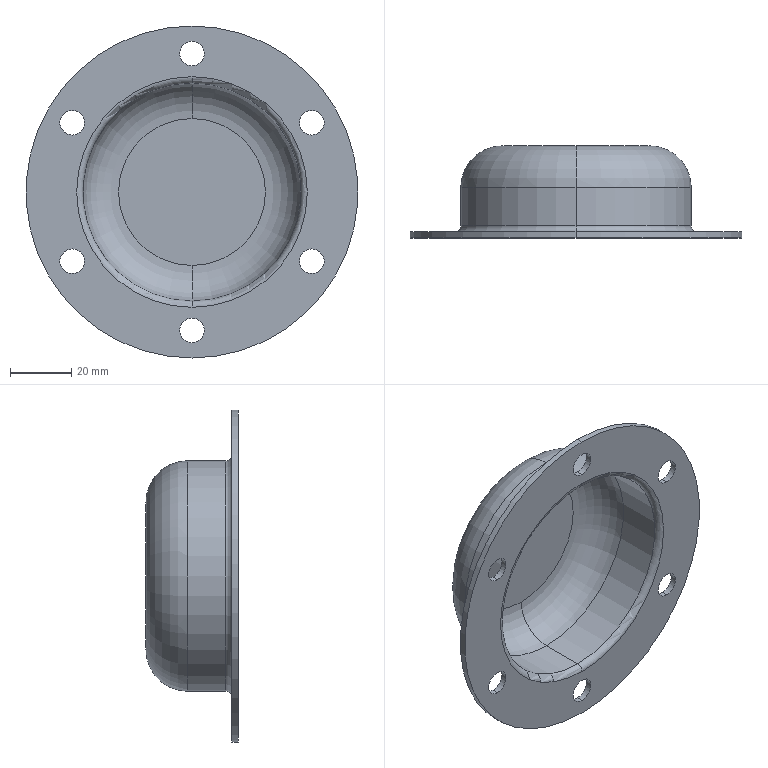Part | SolidWorks | features ICE 1, Revolution 1 | 1 solid | 30 faces | box 108 x 30 x 108 mm | volume 27953 mm3 | cylinder 18 | torus 8 | plane 4 | commonest cylinder face diameters 8 x12 71 x2 75 x2 108 x2
STEP:
#1=CARTESIAN_POINT('',(0.,-15.,-41.));
#2=VERTEX_POINT('',#1);
#3=CARTESIAN_POINT('',(0.,-15.,-49.));
#4=VERTEX_POINT('',#3);
#5=CARTESIAN_POINT('',(0.,-15.,-45.));
#6=DIRECTION('',(0.,-1.,0.));
#7=DIRECTION('',(0.,0.,-1.));
#8=AXIS2_PLACEMENT_3D('',#5,#6,#7);
#9=CIRCLE('',#8,4.);
#10=EDGE_CURVE('',#2,#4,#9,.T.);
#11=ORIENTED_EDGE('',*,*,#10,.T.);
#12=CARTESIAN_POINT('',(0.,-13.,-49.));
#13=VERTEX_POINT('',#12);
#14=CARTESIAN_POINT('',(0.,-23.,-49.));
#15=DIRECTION('',(0.,1.,0.));
#16=VECTOR('',#15,1000.);
#17=LINE('',#14,#16);
#18=EDGE_CURVE('',#4,#13,#17,.T.);
#19=ORIENTED_EDGE('',*,*,#18,.T.);
#20=CARTESIAN_POINT('',(0.,-13.,-41.));
#21=VERTEX_POINT('',#20);
#22=CARTESIAN_POINT('',(0.,-13.,-45.));
#23=DIRECTION('',(0.,1.,0.));
#24=DIRECTION('',(0.,0.,1.));
#25=AXIS2_PLACEMENT_3D('',#22,#23,#24);
#26=CIRCLE('',#25,4.);
#27=EDGE_CURVE('',#13,#21,#26,.T.);
#28=ORIENTED_EDGE('',*,*,#27,.T.);
#29=CARTESIAN_POINT('',(0.,-23.,-41.));
#30=DIRECTION('',(0.,1.,0.));
#31=VECTOR('',#30,1000.);
#32=LINE('',#29,#31);
#33=EDGE_CURVE('',#2,#21,#32,.T.);
#34=ORIENTED_EDGE('',*,*,#33,.F.);
#35=EDGE_LOOP('',(#11,#19,#28,#34));
#36=FACE_OUTER_BOUND('',#35,.T.);
#37=CARTESIAN_POINT('',(0.,-23.,-45.));
#38=DIRECTION('',(0.,1.,0.));
#39=DIRECTION('',(0.,0.,1.));
#40=AXIS2_PLACEMENT_3D('',#37,#38,#39);
#41=CYLINDRICAL_SURFACE('',#40,4.);
#42=ADVANCED_FACE('',(#36),#41,.F.);
#43=CARTESIAN_POINT('',(-38.971,-15.,-18.5));
#44=VERTEX_POINT('',#43);
#45=CARTESIAN_POINT('',(-38.971,-15.,-26.5));
#46=VERTEX_POINT('',#45);
#47=CARTESIAN_POINT('',(-38.971,-15.,-22.5));
#48=DIRECTION('',(0.,-1.,0.));
#49=DIRECTION('',(0.,0.,-1.));
#50=AXIS2_PLACEMENT_3D('',#47,#48,#49);
#51=CIRCLE('',#50,4.);
#52=EDGE_CURVE('',#44,#46,#51,.T.);
#53=ORIENTED_EDGE('',*,*,#52,.T.);
#54=CARTESIAN_POINT('',(-38.971,-13.,-26.5));
#55=VERTEX_POINT('',#54);
#56=CARTESIAN_POINT('',(-38.971,-23.,-26.5));
#57=DIRECTION('',(0.,1.,0.));
#58=VECTOR('',#57,1000.);
#59=LINE('',#56,#58);
#60=EDGE_CURVE('',#46,#55,#59,.T.);
#61=ORIENTED_EDGE('',*,*,#60,.T.);
#62=CARTESIAN_POINT('',(-38.971,-13.,-18.5));
#63=VERTEX_POINT('',#62);
#64=CARTESIAN_POINT('',(-38.971,-13.,-22.5));
#65=DIRECTION('',(0.,1.,0.));
#66=DIRECTION('',(0.,0.,1.));
#67=AXIS2_PLACEMENT_3D('',#64,#65,#66);
#68=CIRCLE('',#67,4.);
#69=EDGE_CURVE('',#55,#63,#68,.T.);
#70=ORIENTED_EDGE('',*,*,#69,.T.);
#71=CARTESIAN_POINT('',(-38.971,-23.,-18.5));
#72=DIRECTION('',(0.,1.,0.));
#73=VECTOR('',#72,1000.);
#74=LINE('',#71,#73);
#75=EDGE_CURVE('',#44,#63,#74,.T.);
#76=ORIENTED_EDGE('',*,*,#75,.F.);
#77=EDGE_LOOP('',(#53,#61,#70,#76));
#78=FACE_OUTER_BOUND('',#77,.T.);
#79=CARTESIAN_POINT('',(-38.971,-23.,-22.5));
#80=DIRECTION('',(0.,1.,0.));
#81=DIRECTION('',(0.,0.,1.));
#82=AXIS2_PLACEMENT_3D('',#79,#80,#81);
#83=CYLINDRICAL_SURFACE('',#82,4.);
#84=ADVANCED_FACE('',(#78),#83,.F.);
#85=CARTESIAN_POINT('',(-38.971,-15.,26.5));
#86=VERTEX_POINT('',#85);
#87=CARTESIAN_POINT('',(-38.971,-15.,18.5));
#88=VERTEX_POINT('',#87);
#89=CARTESIAN_POINT('',(-38.971,-15.,22.5));
#90=DIRECTION('',(0.,-1.,0.));
#91=DIRECTION('',(0.,0.,-1.));
#92=AXIS2_PLACEMENT_3D('',#89,#90,#91);
#93=CIRCLE('',#92,4.);
#94=EDGE_CURVE('',#86,#88,#93,.T.);
#95=ORIENTED_EDGE('',*,*,#94,.T.);
#96=CARTESIAN_POINT('',(-38.971,-13.,18.5));
#97=VERTEX_POINT('',#96);
#98=CARTESIAN_POINT('',(-38.971,-23.,18.5));
#99=DIRECTION('',(0.,1.,0.));
#100=VECTOR('',#99,1000.);
#101=LINE('',#98,#100);
#102=EDGE_CURVE('',#88,#97,#101,.T.);
#103=ORIENTED_EDGE('',*,*,#102,.T.);
#104=CARTESIAN_POINT('',(-38.971,-13.,26.5));
#105=VERTEX_POINT('',#104);
#106=CARTESIAN_POINT('',(-38.971,-13.,22.5));
#107=DIRECTION('',(0.,1.,0.));
#108=DIRECTION('',(0.,0.,1.));
#109=AXIS2_PLACEMENT_3D('',#106,#107,#108);
#110=CIRCLE('',#109,4.);
#111=EDGE_CURVE('',#97,#105,#110,.T.);
#112=ORIENTED_EDGE('',*,*,#111,.T.);
#113=CARTESIAN_POINT('',(-38.971,-23.,26.5));
#114=DIRECTION('',(0.,1.,0.));
#115=VECTOR('',#114,1000.);
#116=LINE('',#113,#115);
#117=EDGE_CURVE('',#86,#105,#116,.T.);
#118=ORIENTED_EDGE('',*,*,#117,.F.);
#119=EDGE_LOOP('',(#95,#103,#112,#118));
#120=FACE_OUTER_BOUND('',#119,.T.);
#121=CARTESIAN_POINT('',(-38.971,-23.,22.5));
#122=DIRECTION('',(0.,1.,0.));
#123=DIRECTION('',(0.,0.,1.));
#124=AXIS2_PLACEMENT_3D('',#121,#122,#123);
#125=CYLINDRICAL_SURFACE('',#124,4.);
#126=ADVANCED_FACE('',(#120),#125,.F.);
#127=CARTESIAN_POINT('',(0.,-15.,49.));
#128=VERTEX_POINT('',#127);
#129=CARTESIAN_POINT('',(0.,-15.,41.));
#130=VERTEX_POINT('',#129);
#131=CARTESIAN_POINT('',(0.,-15.,45.));
#132=DIRECTION('',(0.,-1.,0.));
#133=DIRECTION('',(0.,0.,-1.));
#134=AXIS2_PLACEMENT_3D('',#131,#132,#133);
#135=CIRCLE('',#134,4.);
#136=EDGE_CURVE('',#128,#130,#135,.T.);
#137=ORIENTED_EDGE('',*,*,#136,.T.);
#138=CARTESIAN_POINT('',(0.,-13.,41.));
#139=VERTEX_POINT('',#138);
#140=CARTESIAN_POINT('',(0.,-23.,41.));
#141=DIRECTION('',(0.,1.,0.));
#142=VECTOR('',#141,1000.);
#143=LINE('',#140,#142);
#144=EDGE_CURVE('',#130,#139,#143,.T.);
#145=ORIENTED_EDGE('',*,*,#144,.T.);
#146=CARTESIAN_POINT('',(0.,-13.,49.));
#147=VERTEX_POINT('',#146);
#148=CARTESIAN_POINT('',(0.,-13.,45.));
#149=DIRECTION('',(0.,1.,0.));
#150=DIRECTION('',(0.,0.,1.));
#151=AXIS2_PLACEMENT_3D('',#148,#149,#150);
#152=CIRCLE('',#151,4.);
#153=EDGE_CURVE('',#139,#147,#152,.T.);
#154=ORIENTED_EDGE('',*,*,#153,.T.);
#155=CARTESIAN_POINT('',(0.,-23.,49.));
#156=DIRECTION('',(0.,1.,0.));
#157=VECTOR('',#156,1000.);
#158=LINE('',#155,#157);
#159=EDGE_CURVE('',#128,#147,#158,.T.);
#160=ORIENTED_EDGE('',*,*,#159,.F.);
#161=EDGE_LOOP('',(#137,#145,#154,#160));
#162=FACE_OUTER_BOUND('',#161,.T.);
#163=CARTESIAN_POINT('',(0.,-23.,45.));
#164=DIRECTION('',(0.,1.,0.));
#165=DIRECTION('',(0.,0.,1.));
#166=AXIS2_PLACEMENT_3D('',#163,#164,#165);
#167=CYLINDRICAL_SURFACE('',#166,4.);
#168=ADVANCED_FACE('',(#162),#167,.F.);
#169=CARTESIAN_POINT('',(38.971,-15.,26.5));
#170=VERTEX_POINT('',#169);
#171=CARTESIAN_POINT('',(38.971,-15.,18.5));
#172=VERTEX_POINT('',#171);
#173=CARTESIAN_POINT('',(38.971,-15.,22.5));
#174=DIRECTION('',(0.,-1.,0.));
#175=DIRECTION('',(0.,0.,-1.));
#176=AXIS2_PLACEMENT_3D('',#173,#174,#175);
#177=CIRCLE('',#176,4.);
#178=EDGE_CURVE('',#170,#172,#177,.T.);
#179=ORIENTED_EDGE('',*,*,#178,.T.);
#180=CARTESIAN_POINT('',(38.971,-13.,18.5));
#181=VERTEX_POINT('',#180);
#182=CARTESIAN_POINT('',(38.971,-23.,18.5));
#183=DIRECTION('',(0.,1.,0.));
#184=VECTOR('',#183,1000.);
#185=LINE('',#182,#184);
#186=EDGE_CURVE('',#172,#181,#185,.T.);
#187=ORIENTED_EDGE('',*,*,#186,.T.);
#188=CARTESIAN_POINT('',(38.971,-13.,26.5));
#189=VERTEX_POINT('',#188);
#190=CARTESIAN_POINT('',(38.971,-13.,22.5));
#191=DIRECTION('',(0.,1.,0.));
#192=DIRECTION('',(0.,0.,1.));
#193=AXIS2_PLACEMENT_3D('',#190,#191,#192);
#194=CIRCLE('',#193,4.);
#195=EDGE_CURVE('',#181,#189,#194,.T.);
#196=ORIENTED_EDGE('',*,*,#195,.T.);
#197=CARTESIAN_POINT('',(38.971,-23.,26.5));
#198=DIRECTION('',(0.,1.,0.));
#199=VECTOR('',#198,1000.);
#200=LINE('',#197,#199);
#201=EDGE_CURVE('',#170,#189,#200,.T.);
#202=ORIENTED_EDGE('',*,*,#201,.F.);
#203=EDGE_LOOP('',(#179,#187,#196,#202));
#204=FACE_OUTER_BOUND('',#203,.T.);
#205=CARTESIAN_POINT('',(38.971,-23.,22.5));
#206=DIRECTION('',(0.,1.,0.));
#207=DIRECTION('',(0.,0.,1.));
#208=AXIS2_PLACEMENT_3D('',#205,#206,#207);
#209=CYLINDRICAL_SURFACE('',#208,4.);
#210=ADVANCED_FACE('',(#204),#209,.F.);
#211=CARTESIAN_POINT('',(38.971,-15.,-18.5));
#212=VERTEX_POINT('',#211);
#213=CARTESIAN_POINT('',(38.971,-15.,-26.5));
#214=VERTEX_POINT('',#213);
#215=CARTESIAN_POINT('',(38.971,-15.,-22.5));
#216=DIRECTION('',(0.,-1.,0.));
#217=DIRECTION('',(0.,0.,-1.));
#218=AXIS2_PLACEMENT_3D('',#215,#216,#217);
#219=CIRCLE('',#218,4.);
#220=EDGE_CURVE('',#212,#214,#219,.T.);
#221=ORIENTED_EDGE('',*,*,#220,.T.);
#222=CARTESIAN_POINT('',(38.971,-13.,-26.5));
#223=VERTEX_POINT('',#222);
#224=CARTESIAN_POINT('',(38.971,-23.,-26.5));
#225=DIRECTION('',(0.,1.,0.));
#226=VECTOR('',#225,1000.);
#227=LINE('',#224,#226);
#228=EDGE_CURVE('',#214,#223,#227,.T.);
#229=ORIENTED_EDGE('',*,*,#228,.T.);
#230=CARTESIAN_POINT('',(38.971,-13.,-18.5));
#231=VERTEX_POINT('',#230);
#232=CARTESIAN_POINT('',(38.971,-13.,-22.5));
#233=DIRECTION('',(0.,1.,0.));
#234=DIRECTION('',(0.,0.,1.));
#235=AXIS2_PLACEMENT_3D('',#232,#233,#234);
#236=CIRCLE('',#235,4.);
#237=EDGE_CURVE('',#223,#231,#236,.T.);
#238=ORIENTED_EDGE('',*,*,#237,.T.);
#239=CARTESIAN_POINT('',(38.971,-23.,-18.5));
#240=DIRECTION('',(0.,1.,0.));
#241=VECTOR('',#240,1000.);
#242=LINE('',#239,#241);
#243=EDGE_CURVE('',#212,#231,#242,.T.);
#244=ORIENTED_EDGE('',*,*,#243,.F.);
#245=EDGE_LOOP('',(#221,#229,#238,#244));
#246=FACE_OUTER_BOUND('',#245,.T.);
#247=CARTESIAN_POINT('',(38.971,-23.,-22.5));
#248=DIRECTION('',(0.,1.,0.));
#249=DIRECTION('',(0.,0.,1.));
#250=AXIS2_PLACEMENT_3D('',#247,#248,#249);
#251=CYLINDRICAL_SURFACE('',#250,4.);
#252=ADVANCED_FACE('',(#246),#251,.F.);
#253=CARTESIAN_POINT('',(0.,1.423,-37.5));
#254=VERTEX_POINT('',#253);
#255=CARTESIAN_POINT('',(0.,1.423,37.5));
#256=VERTEX_POINT('',#255);
#257=CARTESIAN_POINT('',(0.,1.423,0.));
#258=DIRECTION('',(0.,-1.,0.));
#259=DIRECTION('',(0.,0.,-1.));
#260=AXIS2_PLACEMENT_3D('',#257,#258,#259);
#261=CIRCLE('',#260,37.5);
#262=EDGE_CURVE('',#254,#256,#261,.T.);
#263=ORIENTED_EDGE('',*,*,#262,.T.);
#264=CARTESIAN_POINT('',(0.,-11.,37.5));
#265=VERTEX_POINT('',#264);
#266=CARTESIAN_POINT('',(0.,0.,37.5));
#267=DIRECTION('',(0.,-1.,0.));
#268=VECTOR('',#267,1000.);
#269=LINE('',#266,#268);
#270=EDGE_CURVE('',#256,#265,#269,.T.);
#271=ORIENTED_EDGE('',*,*,#270,.T.);
#272=CARTESIAN_POINT('',(0.,-11.,-37.5));
#273=VERTEX_POINT('',#272);
#274=CARTESIAN_POINT('',(0.,-11.,0.));
#275=DIRECTION('',(0.,-1.,0.));
#276=DIRECTION('',(0.,0.,-1.));
#277=AXIS2_PLACEMENT_3D('',#274,#275,#276);
#278=CIRCLE('',#277,37.5);
#279=EDGE_CURVE('',#273,#265,#278,.T.);
#280=ORIENTED_EDGE('',*,*,#279,.F.);
#281=CARTESIAN_POINT('',(0.,0.,-37.5));
#282=DIRECTION('',(0.,-1.,0.));
#283=VECTOR('',#282,1000.);
#284=LINE('',#281,#283);
#285=EDGE_CURVE('',#254,#273,#284,.T.);
#286=ORIENTED_EDGE('',*,*,#285,.F.);
#287=EDGE_LOOP('',(#263,#271,#280,#286));
#288=FACE_OUTER_BOUND('',#287,.T.);
#289=CARTESIAN_POINT('',(0.,0.,0.));
#290=DIRECTION('',(0.,-1.,0.));
#291=DIRECTION('',(0.,0.,-1.));
#292=AXIS2_PLACEMENT_3D('',#289,#290,#291);
#293=CYLINDRICAL_SURFACE('',#292,37.5);
#294=ADVANCED_FACE('',(#288),#293,.T.);
#295=CARTESIAN_POINT('',(0.,-13.,39.5));
#296=VERTEX_POINT('',#295);
#297=CARTESIAN_POINT('',(0.,-13.,-39.5));
#298=VERTEX_POINT('',#297);
#299=CARTESIAN_POINT('',(0.,-13.,0.));
#300=DIRECTION('',(0.,-1.,0.));
#301=DIRECTION('',(0.,0.,-1.));
#302=AXIS2_PLACEMENT_3D('',#299,#300,#301);
#303=CIRCLE('',#302,39.5);
#304=EDGE_CURVE('',#296,#298,#303,.T.);
#305=ORIENTED_EDGE('',*,*,#304,.F.);
#306=CARTESIAN_POINT('',(0.,-11.,39.5));
#307=DIRECTION('',(1.,0.,0.));
#308=DIRECTION('',(0.,0.,-1.));
#309=AXIS2_PLACEMENT_3D('',#306,#307,#308);
#310=CIRCLE('',#309,2.);
#311=EDGE_CURVE('',#296,#265,#310,.T.);
#312=ORIENTED_EDGE('',*,*,#311,.T.);
#313=CARTESIAN_POINT('',(0.,-11.,0.));
#314=DIRECTION('',(0.,-1.,0.));
#315=DIRECTION('',(0.,0.,-1.));
#316=AXIS2_PLACEMENT_3D('',#313,#314,#315);
#317=CIRCLE('',#316,37.5);
#318=EDGE_CURVE('',#265,#273,#317,.T.);
#319=ORIENTED_EDGE('',*,*,#318,.T.);
#320=CARTESIAN_POINT('',(0.,-11.,-39.5));
#321=DIRECTION('',(-1.,0.,0.));
#322=DIRECTION('',(0.,0.,1.));
#323=AXIS2_PLACEMENT_3D('',#320,#321,#322);
#324=CIRCLE('',#323,2.);
#325=EDGE_CURVE('',#298,#273,#324,.T.);
#326=ORIENTED_EDGE('',*,*,#325,.F.);
#327=EDGE_LOOP('',(#305,#312,#319,#326));
#328=FACE_OUTER_BOUND('',#327,.T.);
#329=CARTESIAN_POINT('',(0.,-11.,0.));
#330=DIRECTION('',(0.,-1.,0.));
#331=DIRECTION('',(0.,0.,-1.));
#332=AXIS2_PLACEMENT_3D('',#329,#330,#331);
#333=TOROIDAL_SURFACE('',#332,39.5,2.);
#334=ADVANCED_FACE('',(#328),#333,.F.);
#335=CARTESIAN_POINT('',(0.,-13.,-54.));
#336=VERTEX_POINT('',#335);
#337=CARTESIAN_POINT('',(0.,-13.,54.));
#338=VERTEX_POINT('',#337);
#339=CARTESIAN_POINT('',(0.,-13.,0.));
#340=DIRECTION('',(0.,-1.,0.));
#341=DIRECTION('',(0.,0.,-1.));
#342=AXIS2_PLACEMENT_3D('',#339,#340,#341);
#343=CIRCLE('',#342,54.);
#344=EDGE_CURVE('',#336,#338,#343,.T.);
#345=ORIENTED_EDGE('',*,*,#344,.T.);
#346=CARTESIAN_POINT('',(0.,-15.,54.));
#347=VERTEX_POINT('',#346);
#348=CARTESIAN_POINT('',(0.,0.,54.));
#349=DIRECTION('',(0.,-1.,0.));
#350=VECTOR('',#349,1000.);
#351=LINE('',#348,#350);
#352=EDGE_CURVE('',#338,#347,#351,.T.);
#353=ORIENTED_EDGE('',*,*,#352,.T.);
#354=CARTESIAN_POINT('',(0.,-15.,-54.));
#355=VERTEX_POINT('',#354);
#356=CARTESIAN_POINT('',(0.,-15.,0.));
#357=DIRECTION('',(0.,-1.,0.));
#358=DIRECTION('',(0.,0.,-1.));
#359=AXIS2_PLACEMENT_3D('',#356,#357,#358);
#360=CIRCLE('',#359,54.);
#361=EDGE_CURVE('',#355,#347,#360,.T.);
#362=ORIENTED_EDGE('',*,*,#361,.F.);
#363=CARTESIAN_POINT('',(0.,0.,-54.));
#364=DIRECTION('',(0.,-1.,0.));
#365=VECTOR('',#364,1000.);
#366=LINE('',#363,#365);
#367=EDGE_CURVE('',#336,#355,#366,.T.);
#368=ORIENTED_EDGE('',*,*,#367,.F.);
#369=EDGE_LOOP('',(#345,#353,#362,#368));
#370=FACE_OUTER_BOUND('',#369,.T.);
#371=CARTESIAN_POINT('',(0.,0.,0.));
#372=DIRECTION('',(0.,-1.,0.));
#373=DIRECTION('',(0.,0.,-1.));
#374=AXIS2_PLACEMENT_3D('',#371,#372,#373);
#375=CYLINDRICAL_SURFACE('',#374,54.);
#376=ADVANCED_FACE('',(#370),#375,.T.);
#377=CARTESIAN_POINT('',(0.,-15.,-37.5));
#378=VERTEX_POINT('',#377);
#379=CARTESIAN_POINT('',(0.,-15.,37.5));
#380=VERTEX_POINT('',#379);
#381=CARTESIAN_POINT('',(0.,-15.,0.));
#382=DIRECTION('',(0.,-1.,0.));
#383=DIRECTION('',(0.,0.,-1.));
#384=AXIS2_PLACEMENT_3D('',#381,#382,#383);
#385=CIRCLE('',#384,37.5);
#386=EDGE_CURVE('',#378,#380,#385,.T.);
#387=ORIENTED_EDGE('',*,*,#386,.T.);
#388=CARTESIAN_POINT('',(0.,-13.,35.5));
#389=VERTEX_POINT('',#388);
#390=CARTESIAN_POINT('',(0.,-13.,37.5));
#391=DIRECTION('',(1.,0.,0.));
#392=DIRECTION('',(0.,0.,-1.));
#393=AXIS2_PLACEMENT_3D('',#390,#391,#392);
#394=CIRCLE('',#393,2.);
#395=EDGE_CURVE('',#380,#389,#394,.T.);
#396=ORIENTED_EDGE('',*,*,#395,.T.);
#397=CARTESIAN_POINT('',(0.,-13.,-35.5));
#398=VERTEX_POINT('',#397);
#399=CARTESIAN_POINT('',(0.,-13.,0.));
#400=DIRECTION('',(0.,-1.,0.));
#401=DIRECTION('',(0.,0.,-1.));
#402=AXIS2_PLACEMENT_3D('',#399,#400,#401);
#403=CIRCLE('',#402,35.5);
#404=EDGE_CURVE('',#398,#389,#403,.T.);
#405=ORIENTED_EDGE('',*,*,#404,.F.);
#406=CARTESIAN_POINT('',(0.,-13.,-37.5));
#407=DIRECTION('',(-1.,0.,0.));
#408=DIRECTION('',(0.,0.,1.));
#409=AXIS2_PLACEMENT_3D('',#406,#407,#408);
#410=CIRCLE('',#409,2.);
#411=EDGE_CURVE('',#378,#398,#410,.T.);
#412=ORIENTED_EDGE('',*,*,#411,.F.);
#413=EDGE_LOOP('',(#387,#396,#405,#412));
#414=FACE_OUTER_BOUND('',#413,.T.);
#415=CARTESIAN_POINT('',(0.,-13.,0.));
#416=DIRECTION('',(0.,-1.,0.));
#417=DIRECTION('',(0.,0.,-1.));
#418=AXIS2_PLACEMENT_3D('',#415,#416,#417);
#419=TOROIDAL_SURFACE('',#418,37.5,2.);
#420=ADVANCED_FACE('',(#414),#419,.T.);
#421=CARTESIAN_POINT('',(0.,1.423,35.5));
#422=VERTEX_POINT('',#421);
#423=CARTESIAN_POINT('',(0.,1.423,-35.5));
#424=VERTEX_POINT('',#423);
#425=CARTESIAN_POINT('',(0.,1.423,0.));
#426=DIRECTION('',(0.,-1.,0.));
#427=DIRECTION('',(0.,0.,-1.));
#428=AXIS2_PLACEMENT_3D('',#425,#426,#427);
#429=CIRCLE('',#428,35.5);
#430=EDGE_CURVE('',#422,#424,#429,.T.);
#431=ORIENTED_EDGE('',*,*,#430,.F.);
#432=CARTESIAN_POINT('',(0.,0.,35.5));
#433=DIRECTION('',(0.,-1.,0.));
#434=VECTOR('',#433,1000.);
#435=LINE('',#432,#434);
#436=EDGE_CURVE('',#422,#389,#435,.T.);
#437=ORIENTED_EDGE('',*,*,#436,.T.);
#438=CARTESIAN_POINT('',(0.,-13.,0.));
#439=DIRECTION('',(0.,-1.,0.));
#440=DIRECTION('',(0.,0.,-1.));
#441=AXIS2_PLACEMENT_3D('',#438,#439,#440);
#442=CIRCLE('',#441,35.5);
#443=EDGE_CURVE('',#389,#398,#442,.T.);
#444=ORIENTED_EDGE('',*,*,#443,.T.);
#445=CARTESIAN_POINT('',(0.,0.,-35.5));
#446=DIRECTION('',(0.,-1.,0.));
#447=VECTOR('',#446,1000.);
#448=LINE('',#445,#447);
#449=EDGE_CURVE('',#424,#398,#448,.T.);
#450=ORIENTED_EDGE('',*,*,#449,.F.);
#451=EDGE_LOOP('',(#431,#437,#444,#450));
#452=FACE_OUTER_BOUND('',#451,.T.);
#453=CARTESIAN_POINT('',(0.,0.,0.));
#454=DIRECTION('',(0.,-1.,0.));
#455=DIRECTION('',(0.,0.,-1.));
#456=AXIS2_PLACEMENT_3D('',#453,#454,#455);
#457=CYLINDRICAL_SURFACE('',#456,35.5);
#458=ADVANCED_FACE('',(#452),#457,.F.);
#459=CARTESIAN_POINT('',(0.,13.,23.923));
#460=VERTEX_POINT('',#459);
#461=CARTESIAN_POINT('',(0.,13.,-23.923));
#462=VERTEX_POINT('',#461);
#463=CARTESIAN_POINT('',(0.,13.,0.));
#464=DIRECTION('',(0.,-1.,0.));
#465=DIRECTION('',(0.,0.,-1.));
#466=AXIS2_PLACEMENT_3D('',#463,#464,#465);
#467=CIRCLE('',#466,23.923);
#468=EDGE_CURVE('',#460,#462,#467,.T.);
#469=ORIENTED_EDGE('',*,*,#468,.F.);
#470=CARTESIAN_POINT('',(0.,1.423,23.923));
#471=DIRECTION('',(1.,0.,0.));
#472=DIRECTION('',(0.,0.,-1.));
#473=AXIS2_PLACEMENT_3D('',#470,#471,#472);
#474=CIRCLE('',#473,11.577);
#475=EDGE_CURVE('',#460,#422,#474,.T.);
#476=ORIENTED_EDGE('',*,*,#475,.T.);
#477=ORIENTED_EDGE('',*,*,#430,.T.);
#478=CARTESIAN_POINT('',(0.,1.423,-23.923));
#479=DIRECTION('',(-1.,0.,0.));
#480=DIRECTION('',(0.,0.,1.));
#481=AXIS2_PLACEMENT_3D('',#478,#479,#480);
#482=CIRCLE('',#481,11.577);
#483=EDGE_CURVE('',#462,#424,#482,.T.);
#484=ORIENTED_EDGE('',*,*,#483,.F.);
#485=EDGE_LOOP('',(#469,#476,#477,#484));
#486=FACE_OUTER_BOUND('',#485,.T.);
#487=CARTESIAN_POINT('',(0.,1.423,0.));
#488=DIRECTION('',(0.,-1.,0.));
#489=DIRECTION('',(0.,0.,-1.));
#490=AXIS2_PLACEMENT_3D('',#487,#488,#489);
#491=TOROIDAL_SURFACE('',#490,23.923,11.577);
#492=ADVANCED_FACE('',(#486),#491,.F.);
#493=CARTESIAN_POINT('',(0.,15.,-23.923));
#494=VERTEX_POINT('',#493);
#495=CARTESIAN_POINT('',(0.,15.,23.923));
#496=VERTEX_POINT('',#495);
#497=CARTESIAN_POINT('',(0.,15.,0.));
#498=DIRECTION('',(0.,-1.,0.));
#499=DIRECTION('',(0.,0.,-1.));
#500=AXIS2_PLACEMENT_3D('',#497,#498,#499);
#501=CIRCLE('',#500,23.923);
#502=EDGE_CURVE('',#494,#496,#501,.T.);
#503=ORIENTED_EDGE('',*,*,#502,.T.);
#504=CARTESIAN_POINT('',(0.,1.423,23.923));
#505=DIRECTION('',(1.,0.,0.));
#506=DIRECTION('',(0.,0.,-1.));
#507=AXIS2_PLACEMENT_3D('',#504,#505,#506);
#508=CIRCLE('',#507,13.577);
#509=EDGE_CURVE('',#496,#256,#508,.T.);
#510=ORIENTED_EDGE('',*,*,#509,.T.);
#511=ORIENTED_EDGE('',*,*,#262,.F.);
#512=CARTESIAN_POINT('',(0.,1.423,-23.923));
#513=DIRECTION('',(-1.,0.,0.));
#514=DIRECTION('',(0.,0.,1.));
#515=AXIS2_PLACEMENT_3D('',#512,#513,#514);
#516=CIRCLE('',#515,13.577);
#517=EDGE_CURVE('',#494,#254,#516,.T.);
#518=ORIENTED_EDGE('',*,*,#517,.F.);
#519=EDGE_LOOP('',(#503,#510,#511,#518));
#520=FACE_OUTER_BOUND('',#519,.T.);
#521=CARTESIAN_POINT('',(0.,1.423,0.));
#522=DIRECTION('',(0.,-1.,0.));
#523=DIRECTION('',(0.,0.,-1.));
#524=AXIS2_PLACEMENT_3D('',#521,#522,#523);
#525=TOROIDAL_SURFACE('',#524,23.923,13.577);
#526=ADVANCED_FACE('',(#520),#525,.T.);
#527=ORIENTED_EDGE('',*,*,#509,.F.);
#528=CARTESIAN_POINT('',(0.,15.,0.));
#529=DIRECTION('',(0.,-1.,0.));
#530=DIRECTION('',(0.,0.,-1.));
#531=AXIS2_PLACEMENT_3D('',#528,#529,#530);
#532=CIRCLE('',#531,23.923);
#533=EDGE_CURVE('',#496,#494,#532,.T.);
#534=ORIENTED_EDGE('',*,*,#533,.T.);
#535=ORIENTED_EDGE('',*,*,#517,.T.);
#536=CARTESIAN_POINT('',(0.,1.423,0.));
#537=DIRECTION('',(0.,-1.,0.));
#538=DIRECTION('',(0.,0.,-1.));
#539=AXIS2_PLACEMENT_3D('',#536,#537,#538);
#540=CIRCLE('',#539,37.5);
#541=EDGE_CURVE('',#256,#254,#540,.T.);
#542=ORIENTED_EDGE('',*,*,#541,.F.);
#543=EDGE_LOOP('',(#527,#534,#535,#542));
#544=FACE_OUTER_BOUND('',#543,.T.);
#545=CARTESIAN_POINT('',(0.,1.423,0.));
#546=DIRECTION('',(0.,-1.,0.));
#547=DIRECTION('',(0.,0.,-1.));
#548=AXIS2_PLACEMENT_3D('',#545,#546,#547);
#549=TOROIDAL_SURFACE('',#548,23.923,13.577);
#550=ADVANCED_FACE('',(#544),#549,.T.);
#551=ORIENTED_EDGE('',*,*,#502,.F.);
#552=ORIENTED_EDGE('',*,*,#533,.F.);
#553=EDGE_LOOP('',(#551,#552));
#554=FACE_OUTER_BOUND('',#553,.T.);
#555=CARTESIAN_POINT('',(23.923,15.,0.));
#556=DIRECTION('',(0.,1.,0.));
#557=DIRECTION('',(0.,0.,1.));
#558=AXIS2_PLACEMENT_3D('',#555,#556,#557);
#559=PLANE('',#558);
#560=ADVANCED_FACE('',(#554),#559,.T.);
#561=CARTESIAN_POINT('',(0.,13.,0.));
#562=DIRECTION('',(0.,-1.,0.));
#563=DIRECTION('',(0.,0.,-1.));
#564=AXIS2_PLACEMENT_3D('',#561,#562,#563);
#565=CIRCLE('',#564,23.923);
#566=EDGE_CURVE('',#462,#460,#565,.T.);
#567=ORIENTED_EDGE('',*,*,#566,.T.);
#568=ORIENTED_EDGE('',*,*,#468,.T.);
#569=EDGE_LOOP('',(#567,#568));
#570=FACE_OUTER_BOUND('',#569,.T.);
#571=CARTESIAN_POINT('',(0.,13.,0.));
#572=DIRECTION('',(0.,-1.,0.));
#573=DIRECTION('',(0.,0.,-1.));
#574=AXIS2_PLACEMENT_3D('',#571,#572,#573);
#575=PLANE('',#574);
#576=ADVANCED_FACE('',(#570),#575,.T.);
#577=ORIENTED_EDGE('',*,*,#475,.F.);
#578=ORIENTED_EDGE('',*,*,#566,.F.);
#579=ORIENTED_EDGE('',*,*,#483,.T.);
#580=CARTESIAN_POINT('',(0.,1.423,0.));
#581=DIRECTION('',(0.,-1.,0.));
#582=DIRECTION('',(0.,0.,-1.));
#583=AXIS2_PLACEMENT_3D('',#580,#581,#582);
#584=CIRCLE('',#583,35.5);
#585=EDGE_CURVE('',#424,#422,#584,.T.);
#586=ORIENTED_EDGE('',*,*,#585,.T.);
#587=EDGE_LOOP('',(#577,#578,#579,#586));
#588=FACE_OUTER_BOUND('',#587,.T.);
#589=CARTESIAN_POINT('',(0.,1.423,0.));
#590=DIRECTION('',(0.,-1.,0.));
#591=DIRECTION('',(0.,0.,-1.));
#592=AXIS2_PLACEMENT_3D('',#589,#590,#591);
#593=TOROIDAL_SURFACE('',#592,23.923,11.577);
#594=ADVANCED_FACE('',(#588),#593,.F.);
#595=ORIENTED_EDGE('',*,*,#436,.F.);
#596=ORIENTED_EDGE('',*,*,#585,.F.);
#597=ORIENTED_EDGE('',*,*,#449,.T.);
#598=ORIENTED_EDGE('',*,*,#404,.T.);
#599=EDGE_LOOP('',(#595,#596,#597,#598));
#600=FACE_OUTER_BOUND('',#599,.T.);
#601=CARTESIAN_POINT('',(0.,0.,0.));
#602=DIRECTION('',(0.,-1.,0.));
#603=DIRECTION('',(0.,0.,-1.));
#604=AXIS2_PLACEMENT_3D('',#601,#602,#603);
#605=CYLINDRICAL_SURFACE('',#604,35.5);
#606=ADVANCED_FACE('',(#600),#605,.F.);
#607=ORIENTED_EDGE('',*,*,#395,.F.);
#608=CARTESIAN_POINT('',(0.,-15.,0.));
#609=DIRECTION('',(0.,-1.,0.));
#610=DIRECTION('',(0.,0.,-1.));
#611=AXIS2_PLACEMENT_3D('',#608,#609,#610);
#612=CIRCLE('',#611,37.5);
#613=EDGE_CURVE('',#380,#378,#612,.T.);
#614=ORIENTED_EDGE('',*,*,#613,.T.);
#615=ORIENTED_EDGE('',*,*,#411,.T.);
#616=ORIENTED_EDGE('',*,*,#443,.F.);
#617=EDGE_LOOP('',(#607,#614,#615,#616));
#618=FACE_OUTER_BOUND('',#617,.T.);
#619=CARTESIAN_POINT('',(0.,-13.,0.));
#620=DIRECTION('',(0.,-1.,0.));
#621=DIRECTION('',(0.,0.,-1.));
#622=AXIS2_PLACEMENT_3D('',#619,#620,#621);
#623=TOROIDAL_SURFACE('',#622,37.5,2.);
#624=ADVANCED_FACE('',(#618),#623,.T.);
#625=ORIENTED_EDGE('',*,*,#10,.F.);
#626=CARTESIAN_POINT('',(0.,-15.,-45.));
#627=DIRECTION('',(0.,-1.,0.));
#628=DIRECTION('',(0.,0.,-1.));
#629=AXIS2_PLACEMENT_3D('',#626,#627,#628);
#630=CIRCLE('',#629,4.);
#631=EDGE_CURVE('',#4,#2,#630,.T.);
#632=ORIENTED_EDGE('',*,*,#631,.F.);
#633=EDGE_LOOP('',(#625,#632));
#634=FACE_BOUND('',#633,.T.);
#635=ORIENTED_EDGE('',*,*,#52,.F.);
#636=CARTESIAN_POINT('',(-38.971,-15.,-22.5));
#637=DIRECTION('',(0.,-1.,0.));
#638=DIRECTION('',(0.,0.,-1.));
#639=AXIS2_PLACEMENT_3D('',#636,#637,#638);
#640=CIRCLE('',#639,4.);
#641=EDGE_CURVE('',#46,#44,#640,.T.);
#642=ORIENTED_EDGE('',*,*,#641,.F.);
#643=EDGE_LOOP('',(#635,#642));
#644=FACE_BOUND('',#643,.T.);
#645=ORIENTED_EDGE('',*,*,#94,.F.);
#646=CARTESIAN_POINT('',(-38.971,-15.,22.5));
#647=DIRECTION('',(0.,-1.,0.));
#648=DIRECTION('',(0.,0.,-1.));
#649=AXIS2_PLACEMENT_3D('',#646,#647,#648);
#650=CIRCLE('',#649,4.);
#651=EDGE_CURVE('',#88,#86,#650,.T.);
#652=ORIENTED_EDGE('',*,*,#651,.F.);
#653=EDGE_LOOP('',(#645,#652));
#654=FACE_BOUND('',#653,.T.);
#655=ORIENTED_EDGE('',*,*,#136,.F.);
#656=CARTESIAN_POINT('',(0.,-15.,45.));
#657=DIRECTION('',(0.,-1.,0.));
#658=DIRECTION('',(0.,0.,-1.));
#659=AXIS2_PLACEMENT_3D('',#656,#657,#658);
#660=CIRCLE('',#659,4.);
#661=EDGE_CURVE('',#130,#128,#660,.T.);
#662=ORIENTED_EDGE('',*,*,#661,.F.);
#663=EDGE_LOOP('',(#655,#662));
#664=FACE_BOUND('',#663,.T.);
#665=ORIENTED_EDGE('',*,*,#178,.F.);
#666=CARTESIAN_POINT('',(38.971,-15.,22.5));
#667=DIRECTION('',(0.,-1.,0.));
#668=DIRECTION('',(0.,0.,-1.));
#669=AXIS2_PLACEMENT_3D('',#666,#667,#668);
#670=CIRCLE('',#669,4.);
#671=EDGE_CURVE('',#172,#170,#670,.T.);
#672=ORIENTED_EDGE('',*,*,#671,.F.);
#673=EDGE_LOOP('',(#665,#672));
#674=FACE_BOUND('',#673,.T.);
#675=ORIENTED_EDGE('',*,*,#220,.F.);
#676=CARTESIAN_POINT('',(38.971,-15.,-22.5));
#677=DIRECTION('',(0.,-1.,0.));
#678=DIRECTION('',(0.,0.,-1.));
#679=AXIS2_PLACEMENT_3D('',#676,#677,#678);
#680=CIRCLE('',#679,4.);
#681=EDGE_CURVE('',#214,#212,#680,.T.);
#682=ORIENTED_EDGE('',*,*,#681,.F.);
#683=EDGE_LOOP('',(#675,#682));
#684=FACE_BOUND('',#683,.T.);
#685=ORIENTED_EDGE('',*,*,#361,.T.);
#686=CARTESIAN_POINT('',(0.,-15.,0.));
#687=DIRECTION('',(0.,-1.,0.));
#688=DIRECTION('',(0.,0.,-1.));
#689=AXIS2_PLACEMENT_3D('',#686,#687,#688);
#690=CIRCLE('',#689,54.);
#691=EDGE_CURVE('',#347,#355,#690,.T.);
#692=ORIENTED_EDGE('',*,*,#691,.T.);
#693=EDGE_LOOP('',(#685,#692));
#694=FACE_OUTER_BOUND('',#693,.T.);
#695=ORIENTED_EDGE('',*,*,#386,.F.);
#696=ORIENTED_EDGE('',*,*,#613,.F.);
#697=EDGE_LOOP('',(#695,#696));
#698=FACE_BOUND('',#697,.T.);
#699=CARTESIAN_POINT('',(54.,-15.,0.));
#700=DIRECTION('',(0.,-1.,0.));
#701=DIRECTION('',(0.,0.,-1.));
#702=AXIS2_PLACEMENT_3D('',#699,#700,#701);
#703=PLANE('',#702);
#704=ADVANCED_FACE('',(#634,#644,#654,#664,#674,#684,#694,#698),#703,.T.);
#705=ORIENTED_EDGE('',*,*,#352,.F.);
#706=CARTESIAN_POINT('',(0.,-13.,0.));
#707=DIRECTION('',(0.,-1.,0.));
#708=DIRECTION('',(0.,0.,-1.));
#709=AXIS2_PLACEMENT_3D('',#706,#707,#708);
#710=CIRCLE('',#709,54.);
#711=EDGE_CURVE('',#338,#336,#710,.T.);
#712=ORIENTED_EDGE('',*,*,#711,.T.);
#713=ORIENTED_EDGE('',*,*,#367,.T.);
#714=ORIENTED_EDGE('',*,*,#691,.F.);
#715=EDGE_LOOP('',(#705,#712,#713,#714));
#716=FACE_OUTER_BOUND('',#715,.T.);
#717=CARTESIAN_POINT('',(0.,0.,0.));
#718=DIRECTION('',(0.,-1.,0.));
#719=DIRECTION('',(0.,0.,-1.));
#720=AXIS2_PLACEMENT_3D('',#717,#718,#719);
#721=CYLINDRICAL_SURFACE('',#720,54.);
#722=ADVANCED_FACE('',(#716),#721,.T.);
#723=CARTESIAN_POINT('',(0.,-13.,-45.));
#724=DIRECTION('',(0.,1.,0.));
#725=DIRECTION('',(0.,0.,1.));
#726=AXIS2_PLACEMENT_3D('',#723,#724,#725);
#727=CIRCLE('',#726,4.);
#728=EDGE_CURVE('',#21,#13,#727,.T.);
#729=ORIENTED_EDGE('',*,*,#728,.F.);
#730=ORIENTED_EDGE('',*,*,#27,.F.);
#731=EDGE_LOOP('',(#729,#730));
#732=FACE_BOUND('',#731,.T.);
#733=CARTESIAN_POINT('',(-38.971,-13.,-22.5));
#734=DIRECTION('',(0.,1.,0.));
#735=DIRECTION('',(0.,0.,1.));
#736=AXIS2_PLACEMENT_3D('',#733,#734,#735);
#737=CIRCLE('',#736,4.);
#738=EDGE_CURVE('',#63,#55,#737,.T.);
#739=ORIENTED_EDGE('',*,*,#738,.F.);
#740=ORIENTED_EDGE('',*,*,#69,.F.);
#741=EDGE_LOOP('',(#739,#740));
#742=FACE_BOUND('',#741,.T.);
#743=CARTESIAN_POINT('',(-38.971,-13.,22.5));
#744=DIRECTION('',(0.,1.,0.));
#745=DIRECTION('',(0.,0.,1.));
#746=AXIS2_PLACEMENT_3D('',#743,#744,#745);
#747=CIRCLE('',#746,4.);
#748=EDGE_CURVE('',#105,#97,#747,.T.);
#749=ORIENTED_EDGE('',*,*,#748,.F.);
#750=ORIENTED_EDGE('',*,*,#111,.F.);
#751=EDGE_LOOP('',(#749,#750));
#752=FACE_BOUND('',#751,.T.);
#753=CARTESIAN_POINT('',(0.,-13.,45.));
#754=DIRECTION('',(0.,1.,0.));
#755=DIRECTION('',(0.,0.,1.));
#756=AXIS2_PLACEMENT_3D('',#753,#754,#755);
#757=CIRCLE('',#756,4.);
#758=EDGE_CURVE('',#147,#139,#757,.T.);
#759=ORIENTED_EDGE('',*,*,#758,.F.);
#760=ORIENTED_EDGE('',*,*,#153,.F.);
#761=EDGE_LOOP('',(#759,#760));
#762=FACE_BOUND('',#761,.T.);
#763=CARTESIAN_POINT('',(38.971,-13.,22.5));
#764=DIRECTION('',(0.,1.,0.));
#765=DIRECTION('',(0.,0.,1.));
#766=AXIS2_PLACEMENT_3D('',#763,#764,#765);
#767=CIRCLE('',#766,4.);
#768=EDGE_CURVE('',#189,#181,#767,.T.);
#769=ORIENTED_EDGE('',*,*,#768,.F.);
#770=ORIENTED_EDGE('',*,*,#195,.F.);
#771=EDGE_LOOP('',(#769,#770));
#772=FACE_BOUND('',#771,.T.);
#773=CARTESIAN_POINT('',(38.971,-13.,-22.5));
#774=DIRECTION('',(0.,1.,0.));
#775=DIRECTION('',(0.,0.,1.));
#776=AXIS2_PLACEMENT_3D('',#773,#774,#775);
#777=CIRCLE('',#776,4.);
#778=EDGE_CURVE('',#231,#223,#777,.T.);
#779=ORIENTED_EDGE('',*,*,#778,.F.);
#780=ORIENTED_EDGE('',*,*,#237,.F.);
#781=EDGE_LOOP('',(#779,#780));
#782=FACE_BOUND('',#781,.T.);
#783=CARTESIAN_POINT('',(0.,-13.,0.));
#784=DIRECTION('',(0.,-1.,0.));
#785=DIRECTION('',(0.,0.,-1.));
#786=AXIS2_PLACEMENT_3D('',#783,#784,#785);
#787=CIRCLE('',#786,39.5);
#788=EDGE_CURVE('',#298,#296,#787,.T.);
#789=ORIENTED_EDGE('',*,*,#788,.T.);
#790=ORIENTED_EDGE('',*,*,#304,.T.);
#791=EDGE_LOOP('',(#789,#790));
#792=FACE_BOUND('',#791,.T.);
#793=ORIENTED_EDGE('',*,*,#344,.F.);
#794=ORIENTED_EDGE('',*,*,#711,.F.);
#795=EDGE_LOOP('',(#793,#794));
#796=FACE_OUTER_BOUND('',#795,.T.);
#797=CARTESIAN_POINT('',(54.,-13.,0.));
#798=DIRECTION('',(0.,1.,0.));
#799=DIRECTION('',(0.,0.,1.));
#800=AXIS2_PLACEMENT_3D('',#797,#798,#799);
#801=PLANE('',#800);
#802=ADVANCED_FACE('',(#732,#742,#752,#762,#772,#782,#792,#796),#801,.T.);
#803=ORIENTED_EDGE('',*,*,#311,.F.);
#804=ORIENTED_EDGE('',*,*,#788,.F.);
#805=ORIENTED_EDGE('',*,*,#325,.T.);
#806=ORIENTED_EDGE('',*,*,#279,.T.);
#807=EDGE_LOOP('',(#803,#804,#805,#806));
#808=FACE_OUTER_BOUND('',#807,.T.);
#809=CARTESIAN_POINT('',(0.,-11.,0.));
#810=DIRECTION('',(0.,-1.,0.));
#811=DIRECTION('',(0.,0.,-1.));
#812=AXIS2_PLACEMENT_3D('',#809,#810,#811);
#813=TOROIDAL_SURFACE('',#812,39.5,2.);
#814=ADVANCED_FACE('',(#808),#813,.F.);
#815=ORIENTED_EDGE('',*,*,#270,.F.);
#816=ORIENTED_EDGE('',*,*,#541,.T.);
#817=ORIENTED_EDGE('',*,*,#285,.T.);
#818=ORIENTED_EDGE('',*,*,#318,.F.);
#819=EDGE_LOOP('',(#815,#816,#817,#818));
#820=FACE_OUTER_BOUND('',#819,.T.);
#821=CARTESIAN_POINT('',(0.,0.,0.));
#822=DIRECTION('',(0.,-1.,0.));
#823=DIRECTION('',(0.,0.,-1.));
#824=AXIS2_PLACEMENT_3D('',#821,#822,#823);
#825=CYLINDRICAL_SURFACE('',#824,37.5);
#826=ADVANCED_FACE('',(#820),#825,.T.);
#827=ORIENTED_EDGE('',*,*,#228,.F.);
#828=ORIENTED_EDGE('',*,*,#681,.T.);
#829=ORIENTED_EDGE('',*,*,#243,.T.);
#830=ORIENTED_EDGE('',*,*,#778,.T.);
#831=EDGE_LOOP('',(#827,#828,#829,#830));
#832=FACE_OUTER_BOUND('',#831,.T.);
#833=CARTESIAN_POINT('',(38.971,-23.,-22.5));
#834=DIRECTION('',(0.,1.,0.));
#835=DIRECTION('',(0.,0.,1.));
#836=AXIS2_PLACEMENT_3D('',#833,#834,#835);
#837=CYLINDRICAL_SURFACE('',#836,4.);
#838=ADVANCED_FACE('',(#832),#837,.F.);
#839=ORIENTED_EDGE('',*,*,#186,.F.);
#840=ORIENTED_EDGE('',*,*,#671,.T.);
#841=ORIENTED_EDGE('',*,*,#201,.T.);
#842=ORIENTED_EDGE('',*,*,#768,.T.);
#843=EDGE_LOOP('',(#839,#840,#841,#842));
#844=FACE_OUTER_BOUND('',#843,.T.);
#845=CARTESIAN_POINT('',(38.971,-23.,22.5));
#846=DIRECTION('',(0.,1.,0.));
#847=DIRECTION('',(0.,0.,1.));
#848=AXIS2_PLACEMENT_3D('',#845,#846,#847);
#849=CYLINDRICAL_SURFACE('',#848,4.);
#850=ADVANCED_FACE('',(#844),#849,.F.);
#851=ORIENTED_EDGE('',*,*,#144,.F.);
#852=ORIENTED_EDGE('',*,*,#661,.T.);
#853=ORIENTED_EDGE('',*,*,#159,.T.);
#854=ORIENTED_EDGE('',*,*,#758,.T.);
#855=EDGE_LOOP('',(#851,#852,#853,#854));
#856=FACE_OUTER_BOUND('',#855,.T.);
#857=CARTESIAN_POINT('',(0.,-23.,45.));
#858=DIRECTION('',(0.,1.,0.));
#859=DIRECTION('',(0.,0.,1.));
#860=AXIS2_PLACEMENT_3D('',#857,#858,#859);
#861=CYLINDRICAL_SURFACE('',#860,4.);
#862=ADVANCED_FACE('',(#856),#861,.F.);
#863=ORIENTED_EDGE('',*,*,#102,.F.);
#864=ORIENTED_EDGE('',*,*,#651,.T.);
#865=ORIENTED_EDGE('',*,*,#117,.T.);
#866=ORIENTED_EDGE('',*,*,#748,.T.);
#867=EDGE_LOOP('',(#863,#864,#865,#866));
#868=FACE_OUTER_BOUND('',#867,.T.);
#869=CARTESIAN_POINT('',(-38.971,-23.,22.5));
#870=DIRECTION('',(0.,1.,0.));
#871=DIRECTION('',(0.,0.,1.));
#872=AXIS2_PLACEMENT_3D('',#869,#870,#871);
#873=CYLINDRICAL_SURFACE('',#872,4.);
#874=ADVANCED_FACE('',(#868),#873,.F.);
#875=ORIENTED_EDGE('',*,*,#60,.F.);
#876=ORIENTED_EDGE('',*,*,#641,.T.);
#877=ORIENTED_EDGE('',*,*,#75,.T.);
#878=ORIENTED_EDGE('',*,*,#738,.T.);
#879=EDGE_LOOP('',(#875,#876,#877,#878));
#880=FACE_OUTER_BOUND('',#879,.T.);
#881=CARTESIAN_POINT('',(-38.971,-23.,-22.5));
#882=DIRECTION('',(0.,1.,0.));
#883=DIRECTION('',(0.,0.,1.));
#884=AXIS2_PLACEMENT_3D('',#881,#882,#883);
#885=CYLINDRICAL_SURFACE('',#884,4.);
#886=ADVANCED_FACE('',(#880),#885,.F.);
#887=ORIENTED_EDGE('',*,*,#18,.F.);
#888=ORIENTED_EDGE('',*,*,#631,.T.);
#889=ORIENTED_EDGE('',*,*,#33,.T.);
#890=ORIENTED_EDGE('',*,*,#728,.T.);
#891=EDGE_LOOP('',(#887,#888,#889,#890));
#892=FACE_OUTER_BOUND('',#891,.T.);
#893=CARTESIAN_POINT('',(0.,-23.,-45.));
#894=DIRECTION('',(0.,1.,0.));
#895=DIRECTION('',(0.,0.,1.));
#896=AXIS2_PLACEMENT_3D('',#893,#894,#895);
#897=CYLINDRICAL_SURFACE('',#896,4.);
#898=ADVANCED_FACE('',(#892),#897,.F.);
#899=CLOSED_SHELL('',(#42,#84,#126,#168,#210,#252,#294,#334,#376,#420,#458,#492,#526,#550,#560,#576,#594,#606,#624,#704,#722,#802,#814,#826,#838,#850,#862,#874,#886,#898));
#900=MANIFOLD_SOLID_BREP('',#899);
#901=CARTESIAN_POINT('',(0.,0.,0.));
#902=DIRECTION('',(0.,0.,1.));
#903=DIRECTION('',(1.,0.,0.));
#904=AXIS2_PLACEMENT_3D('',#901,#902,#903);
#905=(LENGTH_UNIT()NAMED_UNIT(*)SI_UNIT(.MILLI.,.METRE.));
#906=UNCERTAINTY_MEASURE_WITH_UNIT(LENGTH_MEASURE(0.00001),#905,'','');
#907=(NAMED_UNIT(*)PLANE_ANGLE_UNIT()SI_UNIT($,.RADIAN.));
#908=(NAMED_UNIT(*)SI_UNIT($,.STERADIAN.)SOLID_ANGLE_UNIT());
#909=(GEOMETRIC_REPRESENTATION_CONTEXT(3)GLOBAL_UNCERTAINTY_ASSIGNED_CONTEXT((#906))GLOBAL_UNIT_ASSIGNED_CONTEXT((#905,#907,#908))REPRESENTATION_CONTEXT('',''));
#910=ADVANCED_BREP_SHAPE_REPRESENTATION('',(#900,#904),#909);